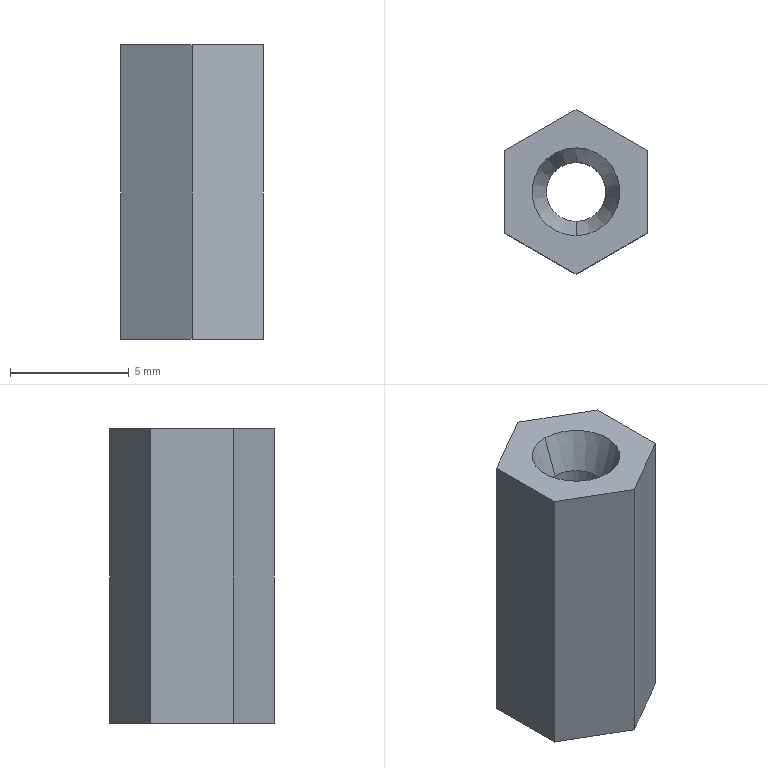Part | STEP file | TQ-DD-1105-THNuts1010_デフォルト | 1 solid | 14 faces | box 6 x 6.928 x 12.4 mm | volume 316.696 mm3 | plane 8 | cone 4 | cylinder 2 | commonest cylinder face diameters 2.5 x2
STEP:
#1=CARTESIAN_POINT('',(0.,1.25,10.75));
#2=VERTEX_POINT('',#1);
#3=CARTESIAN_POINT('',(-1.25,0.,10.75));
#4=VERTEX_POINT('',#3);
#5=CARTESIAN_POINT('',(0.,0.,10.75));
#6=DIRECTION('',(0.,0.,1.));
#7=DIRECTION('',(1.,0.,0.));
#8=AXIS2_PLACEMENT_3D('',#5,#6,#7);
#9=CIRCLE('',#8,1.25);
#10=EDGE_CURVE('',#2,#4,#9,.T.);
#11=ORIENTED_EDGE('',*,*,#10,.F.);
#12=CARTESIAN_POINT('',(0.,1.851,12.4));
#13=VERTEX_POINT('',#12);
#14=CARTESIAN_POINT('',(0.,1.851,12.4));
#15=DIRECTION('',(0.,0.342,0.9397));
#16=VECTOR('',#15,1000.);
#17=LINE('',#14,#16);
#18=EDGE_CURVE('',#2,#13,#17,.T.);
#19=ORIENTED_EDGE('',*,*,#18,.T.);
#20=CARTESIAN_POINT('',(0.,-1.851,12.4));
#21=VERTEX_POINT('',#20);
#22=CARTESIAN_POINT('',(0.,0.,12.4));
#23=DIRECTION('',(0.,0.,-1.));
#24=DIRECTION('',(0.,-1.,0.));
#25=AXIS2_PLACEMENT_3D('',#22,#23,#24);
#26=CIRCLE('',#25,1.851);
#27=EDGE_CURVE('',#21,#13,#26,.T.);
#28=ORIENTED_EDGE('',*,*,#27,.F.);
#29=CARTESIAN_POINT('',(0.,-1.25,10.75));
#30=VERTEX_POINT('',#29);
#31=CARTESIAN_POINT('',(0.,-1.851,12.4));
#32=DIRECTION('',(0.,-0.342,0.9397));
#33=VECTOR('',#32,1000.);
#34=LINE('',#31,#33);
#35=EDGE_CURVE('',#30,#21,#34,.T.);
#36=ORIENTED_EDGE('',*,*,#35,.F.);
#37=CARTESIAN_POINT('',(0.,0.,10.75));
#38=DIRECTION('',(0.,0.,1.));
#39=DIRECTION('',(1.,0.,0.));
#40=AXIS2_PLACEMENT_3D('',#37,#38,#39);
#41=CIRCLE('',#40,1.25);
#42=EDGE_CURVE('',#4,#30,#41,.T.);
#43=ORIENTED_EDGE('',*,*,#42,.F.);
#44=EDGE_LOOP('',(#11,#19,#28,#36,#43));
#45=FACE_OUTER_BOUND('',#44,.T.);
#46=CARTESIAN_POINT('',(0.,0.,12.4));
#47=DIRECTION('',(0.,0.,1.));
#48=DIRECTION('',(0.,-1.,0.));
#49=AXIS2_PLACEMENT_3D('',#46,#47,#48);
#50=CONICAL_SURFACE('',#49,1.851,0.3491);
#51=ADVANCED_FACE('',(#45),#50,.F.);
#52=CARTESIAN_POINT('',(0.,-1.25,1.65));
#53=VERTEX_POINT('',#52);
#54=CARTESIAN_POINT('',(-1.25,0.,1.65));
#55=VERTEX_POINT('',#54);
#56=CARTESIAN_POINT('',(0.,0.,1.65));
#57=DIRECTION('',(0.,0.,-1.));
#58=DIRECTION('',(-0.3242,-0.946,0.));
#59=AXIS2_PLACEMENT_3D('',#56,#57,#58);
#60=CIRCLE('',#59,1.25);
#61=EDGE_CURVE('',#53,#55,#60,.T.);
#62=ORIENTED_EDGE('',*,*,#61,.F.);
#63=CARTESIAN_POINT('',(0.,-1.851,0.));
#64=VERTEX_POINT('',#63);
#65=CARTESIAN_POINT('',(0.,-1.851,0.));
#66=DIRECTION('',(0.,-0.342,-0.9397));
#67=VECTOR('',#66,1000.);
#68=LINE('',#65,#67);
#69=EDGE_CURVE('',#53,#64,#68,.T.);
#70=ORIENTED_EDGE('',*,*,#69,.T.);
#71=CARTESIAN_POINT('',(0.,1.851,0.));
#72=VERTEX_POINT('',#71);
#73=CARTESIAN_POINT('',(0.,0.,0.));
#74=DIRECTION('',(0.,0.,-1.));
#75=DIRECTION('',(0.,1.,0.));
#76=AXIS2_PLACEMENT_3D('',#73,#74,#75);
#77=CIRCLE('',#76,1.851);
#78=EDGE_CURVE('',#64,#72,#77,.T.);
#79=ORIENTED_EDGE('',*,*,#78,.T.);
#80=CARTESIAN_POINT('',(0.,1.25,1.65));
#81=VERTEX_POINT('',#80);
#82=CARTESIAN_POINT('',(0.,1.851,0.));
#83=DIRECTION('',(0.,0.342,-0.9397));
#84=VECTOR('',#83,1000.);
#85=LINE('',#82,#84);
#86=EDGE_CURVE('',#81,#72,#85,.T.);
#87=ORIENTED_EDGE('',*,*,#86,.F.);
#88=CARTESIAN_POINT('',(0.,0.,1.65));
#89=DIRECTION('',(0.,0.,-1.));
#90=DIRECTION('',(-0.3242,-0.946,0.));
#91=AXIS2_PLACEMENT_3D('',#88,#89,#90);
#92=CIRCLE('',#91,1.25);
#93=EDGE_CURVE('',#55,#81,#92,.T.);
#94=ORIENTED_EDGE('',*,*,#93,.F.);
#95=EDGE_LOOP('',(#62,#70,#79,#87,#94));
#96=FACE_OUTER_BOUND('',#95,.T.);
#97=CARTESIAN_POINT('',(0.,0.,0.));
#98=DIRECTION('',(0.,0.,-1.));
#99=DIRECTION('',(0.,1.,0.));
#100=AXIS2_PLACEMENT_3D('',#97,#98,#99);
#101=CONICAL_SURFACE('',#100,1.851,0.3491);
#102=ADVANCED_FACE('',(#96),#101,.F.);
#103=ORIENTED_EDGE('',*,*,#42,.T.);
#104=CARTESIAN_POINT('',(1.25,0.,10.75));
#105=VERTEX_POINT('',#104);
#106=CARTESIAN_POINT('',(0.,0.,10.75));
#107=DIRECTION('',(0.,0.,1.));
#108=DIRECTION('',(1.,0.,0.));
#109=AXIS2_PLACEMENT_3D('',#106,#107,#108);
#110=CIRCLE('',#109,1.25);
#111=EDGE_CURVE('',#30,#105,#110,.T.);
#112=ORIENTED_EDGE('',*,*,#111,.T.);
#113=CARTESIAN_POINT('',(1.25,0.,1.65));
#114=VERTEX_POINT('',#113);
#115=CARTESIAN_POINT('',(1.25,0.,6.86));
#116=DIRECTION('',(0.,0.,-1.));
#117=VECTOR('',#116,1000.);
#118=LINE('',#115,#117);
#119=EDGE_CURVE('',#105,#114,#118,.T.);
#120=ORIENTED_EDGE('',*,*,#119,.T.);
#121=CARTESIAN_POINT('',(0.,0.,1.65));
#122=DIRECTION('',(0.,0.,-1.));
#123=DIRECTION('',(-0.3242,-0.946,0.));
#124=AXIS2_PLACEMENT_3D('',#121,#122,#123);
#125=CIRCLE('',#124,1.25);
#126=EDGE_CURVE('',#114,#53,#125,.T.);
#127=ORIENTED_EDGE('',*,*,#126,.T.);
#128=ORIENTED_EDGE('',*,*,#61,.T.);
#129=CARTESIAN_POINT('',(-1.25,0.,6.86));
#130=DIRECTION('',(0.,0.,-1.));
#131=VECTOR('',#130,1000.);
#132=LINE('',#129,#131);
#133=EDGE_CURVE('',#4,#55,#132,.T.);
#134=ORIENTED_EDGE('',*,*,#133,.F.);
#135=EDGE_LOOP('',(#103,#112,#120,#127,#128,#134));
#136=FACE_OUTER_BOUND('',#135,.T.);
#137=CARTESIAN_POINT('',(0.,0.,6.86));
#138=DIRECTION('',(0.,0.,-1.));
#139=DIRECTION('',(-1.,0.,0.));
#140=AXIS2_PLACEMENT_3D('',#137,#138,#139);
#141=CYLINDRICAL_SURFACE('',#140,1.25);
#142=ADVANCED_FACE('',(#136),#141,.F.);
#143=CARTESIAN_POINT('',(3.,1.732,0.));
#144=VERTEX_POINT('',#143);
#145=CARTESIAN_POINT('',(3.,1.732,12.4));
#146=VERTEX_POINT('',#145);
#147=CARTESIAN_POINT('',(3.,1.732,0.));
#148=DIRECTION('',(0.,0.,1.));
#149=VECTOR('',#148,1000.);
#150=LINE('',#147,#149);
#151=EDGE_CURVE('',#144,#146,#150,.T.);
#152=ORIENTED_EDGE('',*,*,#151,.T.);
#153=CARTESIAN_POINT('',(3.,-1.732,12.4));
#154=VERTEX_POINT('',#153);
#155=CARTESIAN_POINT('',(3.,-1.732,12.4));
#156=DIRECTION('',(0.,-1.,0.));
#157=VECTOR('',#156,1000.);
#158=LINE('',#155,#157);
#159=EDGE_CURVE('',#146,#154,#158,.T.);
#160=ORIENTED_EDGE('',*,*,#159,.T.);
#161=CARTESIAN_POINT('',(3.,-1.732,0.));
#162=VERTEX_POINT('',#161);
#163=CARTESIAN_POINT('',(3.,-1.732,0.));
#164=DIRECTION('',(0.,0.,-1.));
#165=VECTOR('',#164,1000.);
#166=LINE('',#163,#165);
#167=EDGE_CURVE('',#154,#162,#166,.T.);
#168=ORIENTED_EDGE('',*,*,#167,.T.);
#169=CARTESIAN_POINT('',(3.,-1.732,0.));
#170=DIRECTION('',(0.,1.,0.));
#171=VECTOR('',#170,1000.);
#172=LINE('',#169,#171);
#173=EDGE_CURVE('',#162,#144,#172,.T.);
#174=ORIENTED_EDGE('',*,*,#173,.T.);
#175=EDGE_LOOP('',(#152,#160,#168,#174));
#176=FACE_OUTER_BOUND('',#175,.T.);
#177=CARTESIAN_POINT('',(3.,-1.732,0.));
#178=DIRECTION('',(1.,0.,0.));
#179=DIRECTION('',(0.,0.,-1.));
#180=AXIS2_PLACEMENT_3D('',#177,#178,#179);
#181=PLANE('',#180);
#182=ADVANCED_FACE('',(#176),#181,.T.);
#183=ORIENTED_EDGE('',*,*,#27,.T.);
#184=CARTESIAN_POINT('',(0.,0.,12.4));
#185=DIRECTION('',(0.,0.,-1.));
#186=DIRECTION('',(0.,-1.,0.));
#187=AXIS2_PLACEMENT_3D('',#184,#185,#186);
#188=CIRCLE('',#187,1.851);
#189=EDGE_CURVE('',#13,#21,#188,.T.);
#190=ORIENTED_EDGE('',*,*,#189,.T.);
#191=EDGE_LOOP('',(#183,#190));
#192=FACE_BOUND('',#191,.T.);
#193=CARTESIAN_POINT('',(-3.,1.732,12.4));
#194=VERTEX_POINT('',#193);
#195=CARTESIAN_POINT('',(-3.,-1.732,12.4));
#196=VERTEX_POINT('',#195);
#197=CARTESIAN_POINT('',(-3.,0.,12.4));
#198=DIRECTION('',(0.,-1.,0.));
#199=VECTOR('',#198,1000.);
#200=LINE('',#197,#199);
#201=EDGE_CURVE('',#194,#196,#200,.T.);
#202=ORIENTED_EDGE('',*,*,#201,.T.);
#203=CARTESIAN_POINT('',(0.,-3.464,12.4));
#204=VERTEX_POINT('',#203);
#205=CARTESIAN_POINT('',(-3.,-1.732,12.4));
#206=DIRECTION('',(0.866,-0.5,0.));
#207=VECTOR('',#206,1000.);
#208=LINE('',#205,#207);
#209=EDGE_CURVE('',#196,#204,#208,.T.);
#210=ORIENTED_EDGE('',*,*,#209,.T.);
#211=CARTESIAN_POINT('',(0.,-3.464,12.4));
#212=DIRECTION('',(0.866,0.5,0.));
#213=VECTOR('',#212,1000.);
#214=LINE('',#211,#213);
#215=EDGE_CURVE('',#204,#154,#214,.T.);
#216=ORIENTED_EDGE('',*,*,#215,.T.);
#217=ORIENTED_EDGE('',*,*,#159,.F.);
#218=CARTESIAN_POINT('',(0.,3.464,12.4));
#219=VERTEX_POINT('',#218);
#220=CARTESIAN_POINT('',(3.,1.732,12.4));
#221=DIRECTION('',(-0.866,0.5,0.));
#222=VECTOR('',#221,1000.);
#223=LINE('',#220,#222);
#224=EDGE_CURVE('',#146,#219,#223,.T.);
#225=ORIENTED_EDGE('',*,*,#224,.T.);
#226=CARTESIAN_POINT('',(0.,3.464,12.4));
#227=DIRECTION('',(-0.866,-0.5,0.));
#228=VECTOR('',#227,1000.);
#229=LINE('',#226,#228);
#230=EDGE_CURVE('',#219,#194,#229,.T.);
#231=ORIENTED_EDGE('',*,*,#230,.T.);
#232=EDGE_LOOP('',(#202,#210,#216,#217,#225,#231));
#233=FACE_OUTER_BOUND('',#232,.T.);
#234=CARTESIAN_POINT('',(0.,0.,12.4));
#235=DIRECTION('',(0.,0.,1.));
#236=DIRECTION('',(1.,0.,0.));
#237=AXIS2_PLACEMENT_3D('',#234,#235,#236);
#238=PLANE('',#237);
#239=ADVANCED_FACE('',(#192,#233),#238,.T.);
#240=CARTESIAN_POINT('',(0.,3.464,0.));
#241=VERTEX_POINT('',#240);
#242=CARTESIAN_POINT('',(0.,3.464,0.));
#243=DIRECTION('',(0.866,-0.5,0.));
#244=VECTOR('',#243,1000.);
#245=LINE('',#242,#244);
#246=EDGE_CURVE('',#241,#144,#245,.T.);
#247=ORIENTED_EDGE('',*,*,#246,.F.);
#248=CARTESIAN_POINT('',(0.,3.464,0.));
#249=DIRECTION('',(0.,0.,-1.));
#250=VECTOR('',#249,1000.);
#251=LINE('',#248,#250);
#252=EDGE_CURVE('',#219,#241,#251,.T.);
#253=ORIENTED_EDGE('',*,*,#252,.F.);
#254=ORIENTED_EDGE('',*,*,#224,.F.);
#255=ORIENTED_EDGE('',*,*,#151,.F.);
#256=EDGE_LOOP('',(#247,#253,#254,#255));
#257=FACE_OUTER_BOUND('',#256,.T.);
#258=CARTESIAN_POINT('',(0.,3.464,0.));
#259=DIRECTION('',(-0.5,-0.866,0.));
#260=DIRECTION('',(0.866,-0.5,0.));
#261=AXIS2_PLACEMENT_3D('',#258,#259,#260);
#262=PLANE('',#261);
#263=ADVANCED_FACE('',(#257),#262,.F.);
#264=CARTESIAN_POINT('',(0.,0.,0.));
#265=DIRECTION('',(0.,0.,-1.));
#266=DIRECTION('',(0.,1.,0.));
#267=AXIS2_PLACEMENT_3D('',#264,#265,#266);
#268=CIRCLE('',#267,1.851);
#269=EDGE_CURVE('',#72,#64,#268,.T.);
#270=ORIENTED_EDGE('',*,*,#269,.F.);
#271=ORIENTED_EDGE('',*,*,#78,.F.);
#272=EDGE_LOOP('',(#270,#271));
#273=FACE_BOUND('',#272,.T.);
#274=CARTESIAN_POINT('',(-3.,1.732,0.));
#275=VERTEX_POINT('',#274);
#276=CARTESIAN_POINT('',(-3.,-1.732,0.));
#277=VERTEX_POINT('',#276);
#278=CARTESIAN_POINT('',(-3.,0.,0.));
#279=DIRECTION('',(0.,-1.,0.));
#280=VECTOR('',#279,1000.);
#281=LINE('',#278,#280);
#282=EDGE_CURVE('',#275,#277,#281,.T.);
#283=ORIENTED_EDGE('',*,*,#282,.F.);
#284=CARTESIAN_POINT('',(0.,3.464,0.));
#285=DIRECTION('',(-0.866,-0.5,0.));
#286=VECTOR('',#285,1000.);
#287=LINE('',#284,#286);
#288=EDGE_CURVE('',#241,#275,#287,.T.);
#289=ORIENTED_EDGE('',*,*,#288,.F.);
#290=ORIENTED_EDGE('',*,*,#246,.T.);
#291=ORIENTED_EDGE('',*,*,#173,.F.);
#292=CARTESIAN_POINT('',(0.,-3.464,0.));
#293=VERTEX_POINT('',#292);
#294=CARTESIAN_POINT('',(0.,-3.464,0.));
#295=DIRECTION('',(0.866,0.5,0.));
#296=VECTOR('',#295,1000.);
#297=LINE('',#294,#296);
#298=EDGE_CURVE('',#293,#162,#297,.T.);
#299=ORIENTED_EDGE('',*,*,#298,.F.);
#300=CARTESIAN_POINT('',(-3.,-1.732,0.));
#301=DIRECTION('',(0.866,-0.5,0.));
#302=VECTOR('',#301,1000.);
#303=LINE('',#300,#302);
#304=EDGE_CURVE('',#277,#293,#303,.T.);
#305=ORIENTED_EDGE('',*,*,#304,.F.);
#306=EDGE_LOOP('',(#283,#289,#290,#291,#299,#305));
#307=FACE_OUTER_BOUND('',#306,.T.);
#308=CARTESIAN_POINT('',(0.,0.,0.));
#309=DIRECTION('',(0.,0.,1.));
#310=DIRECTION('',(1.,0.,0.));
#311=AXIS2_PLACEMENT_3D('',#308,#309,#310);
#312=PLANE('',#311);
#313=ADVANCED_FACE('',(#273,#307),#312,.F.);
#314=ORIENTED_EDGE('',*,*,#167,.F.);
#315=ORIENTED_EDGE('',*,*,#215,.F.);
#316=CARTESIAN_POINT('',(0.,-3.464,0.));
#317=DIRECTION('',(0.,0.,-1.));
#318=VECTOR('',#317,1000.);
#319=LINE('',#316,#318);
#320=EDGE_CURVE('',#204,#293,#319,.T.);
#321=ORIENTED_EDGE('',*,*,#320,.T.);
#322=ORIENTED_EDGE('',*,*,#298,.T.);
#323=EDGE_LOOP('',(#314,#315,#321,#322));
#324=FACE_OUTER_BOUND('',#323,.T.);
#325=CARTESIAN_POINT('',(0.,-3.464,0.));
#326=DIRECTION('',(0.5,-0.866,0.));
#327=DIRECTION('',(0.866,0.5,0.));
#328=AXIS2_PLACEMENT_3D('',#325,#326,#327);
#329=PLANE('',#328);
#330=ADVANCED_FACE('',(#324),#329,.T.);
#331=ORIENTED_EDGE('',*,*,#18,.F.);
#332=CARTESIAN_POINT('',(0.,0.,10.75));
#333=DIRECTION('',(0.,0.,1.));
#334=DIRECTION('',(1.,0.,0.));
#335=AXIS2_PLACEMENT_3D('',#332,#333,#334);
#336=CIRCLE('',#335,1.25);
#337=EDGE_CURVE('',#105,#2,#336,.T.);
#338=ORIENTED_EDGE('',*,*,#337,.F.);
#339=ORIENTED_EDGE('',*,*,#111,.F.);
#340=ORIENTED_EDGE('',*,*,#35,.T.);
#341=ORIENTED_EDGE('',*,*,#189,.F.);
#342=EDGE_LOOP('',(#331,#338,#339,#340,#341));
#343=FACE_OUTER_BOUND('',#342,.T.);
#344=CARTESIAN_POINT('',(0.,0.,12.4));
#345=DIRECTION('',(0.,0.,1.));
#346=DIRECTION('',(0.,-1.,0.));
#347=AXIS2_PLACEMENT_3D('',#344,#345,#346);
#348=CONICAL_SURFACE('',#347,1.851,0.3491);
#349=ADVANCED_FACE('',(#343),#348,.F.);
#350=CARTESIAN_POINT('',(-3.,-1.732,0.));
#351=DIRECTION('',(0.,0.,1.));
#352=VECTOR('',#351,1000.);
#353=LINE('',#350,#352);
#354=EDGE_CURVE('',#277,#196,#353,.T.);
#355=ORIENTED_EDGE('',*,*,#354,.F.);
#356=ORIENTED_EDGE('',*,*,#304,.T.);
#357=ORIENTED_EDGE('',*,*,#320,.F.);
#358=ORIENTED_EDGE('',*,*,#209,.F.);
#359=EDGE_LOOP('',(#355,#356,#357,#358));
#360=FACE_OUTER_BOUND('',#359,.T.);
#361=CARTESIAN_POINT('',(0.,-3.464,0.));
#362=DIRECTION('',(0.5,0.866,0.));
#363=DIRECTION('',(-0.866,0.5,0.));
#364=AXIS2_PLACEMENT_3D('',#361,#362,#363);
#365=PLANE('',#364);
#366=ADVANCED_FACE('',(#360),#365,.F.);
#367=CARTESIAN_POINT('',(-3.,1.732,0.));
#368=DIRECTION('',(0.,0.,1.));
#369=VECTOR('',#368,1000.);
#370=LINE('',#367,#369);
#371=EDGE_CURVE('',#275,#194,#370,.T.);
#372=ORIENTED_EDGE('',*,*,#371,.F.);
#373=ORIENTED_EDGE('',*,*,#282,.T.);
#374=ORIENTED_EDGE('',*,*,#354,.T.);
#375=ORIENTED_EDGE('',*,*,#201,.F.);
#376=EDGE_LOOP('',(#372,#373,#374,#375));
#377=FACE_OUTER_BOUND('',#376,.T.);
#378=CARTESIAN_POINT('',(-3.,-1.732,0.));
#379=DIRECTION('',(1.,0.,0.));
#380=DIRECTION('',(0.,0.,-1.));
#381=AXIS2_PLACEMENT_3D('',#378,#379,#380);
#382=PLANE('',#381);
#383=ADVANCED_FACE('',(#377),#382,.F.);
#384=ORIENTED_EDGE('',*,*,#288,.T.);
#385=ORIENTED_EDGE('',*,*,#371,.T.);
#386=ORIENTED_EDGE('',*,*,#230,.F.);
#387=ORIENTED_EDGE('',*,*,#252,.T.);
#388=EDGE_LOOP('',(#384,#385,#386,#387));
#389=FACE_OUTER_BOUND('',#388,.T.);
#390=CARTESIAN_POINT('',(0.,3.464,0.));
#391=DIRECTION('',(-0.5,0.866,0.));
#392=DIRECTION('',(-0.866,-0.5,0.));
#393=AXIS2_PLACEMENT_3D('',#390,#391,#392);
#394=PLANE('',#393);
#395=ADVANCED_FACE('',(#389),#394,.T.);
#396=ORIENTED_EDGE('',*,*,#69,.F.);
#397=ORIENTED_EDGE('',*,*,#126,.F.);
#398=CARTESIAN_POINT('',(0.,0.,1.65));
#399=DIRECTION('',(0.,0.,-1.));
#400=DIRECTION('',(-0.3242,-0.946,0.));
#401=AXIS2_PLACEMENT_3D('',#398,#399,#400);
#402=CIRCLE('',#401,1.25);
#403=EDGE_CURVE('',#81,#114,#402,.T.);
#404=ORIENTED_EDGE('',*,*,#403,.F.);
#405=ORIENTED_EDGE('',*,*,#86,.T.);
#406=ORIENTED_EDGE('',*,*,#269,.T.);
#407=EDGE_LOOP('',(#396,#397,#404,#405,#406));
#408=FACE_OUTER_BOUND('',#407,.T.);
#409=CARTESIAN_POINT('',(0.,0.,0.));
#410=DIRECTION('',(0.,0.,-1.));
#411=DIRECTION('',(0.,1.,0.));
#412=AXIS2_PLACEMENT_3D('',#409,#410,#411);
#413=CONICAL_SURFACE('',#412,1.851,0.3491);
#414=ADVANCED_FACE('',(#408),#413,.F.);
#415=ORIENTED_EDGE('',*,*,#119,.F.);
#416=ORIENTED_EDGE('',*,*,#337,.T.);
#417=ORIENTED_EDGE('',*,*,#10,.T.);
#418=ORIENTED_EDGE('',*,*,#133,.T.);
#419=ORIENTED_EDGE('',*,*,#93,.T.);
#420=ORIENTED_EDGE('',*,*,#403,.T.);
#421=EDGE_LOOP('',(#415,#416,#417,#418,#419,#420));
#422=FACE_OUTER_BOUND('',#421,.T.);
#423=CARTESIAN_POINT('',(0.,0.,6.86));
#424=DIRECTION('',(0.,0.,-1.));
#425=DIRECTION('',(-1.,0.,0.));
#426=AXIS2_PLACEMENT_3D('',#423,#424,#425);
#427=CYLINDRICAL_SURFACE('',#426,1.25);
#428=ADVANCED_FACE('',(#422),#427,.F.);
#429=CLOSED_SHELL('',(#51,#102,#142,#182,#239,#263,#313,#330,#349,#366,#383,#395,#414,#428));
#430=MANIFOLD_SOLID_BREP('',#429);
#431=CARTESIAN_POINT('',(0.,0.,0.));
#432=DIRECTION('',(0.,0.,1.));
#433=DIRECTION('',(1.,0.,0.));
#434=AXIS2_PLACEMENT_3D('',#431,#432,#433);
#435=(LENGTH_UNIT()NAMED_UNIT(*)SI_UNIT(.MILLI.,.METRE.));
#436=UNCERTAINTY_MEASURE_WITH_UNIT(LENGTH_MEASURE(0.00001),#435,'','');
#437=(NAMED_UNIT(*)PLANE_ANGLE_UNIT()SI_UNIT($,.RADIAN.));
#438=(NAMED_UNIT(*)SI_UNIT($,.STERADIAN.)SOLID_ANGLE_UNIT());
#439=(GEOMETRIC_REPRESENTATION_CONTEXT(3)GLOBAL_UNCERTAINTY_ASSIGNED_CONTEXT((#436))GLOBAL_UNIT_ASSIGNED_CONTEXT((#435,#437,#438))REPRESENTATION_CONTEXT('',''));
#440=ADVANCED_BREP_SHAPE_REPRESENTATION('',(#430,#434),#439);